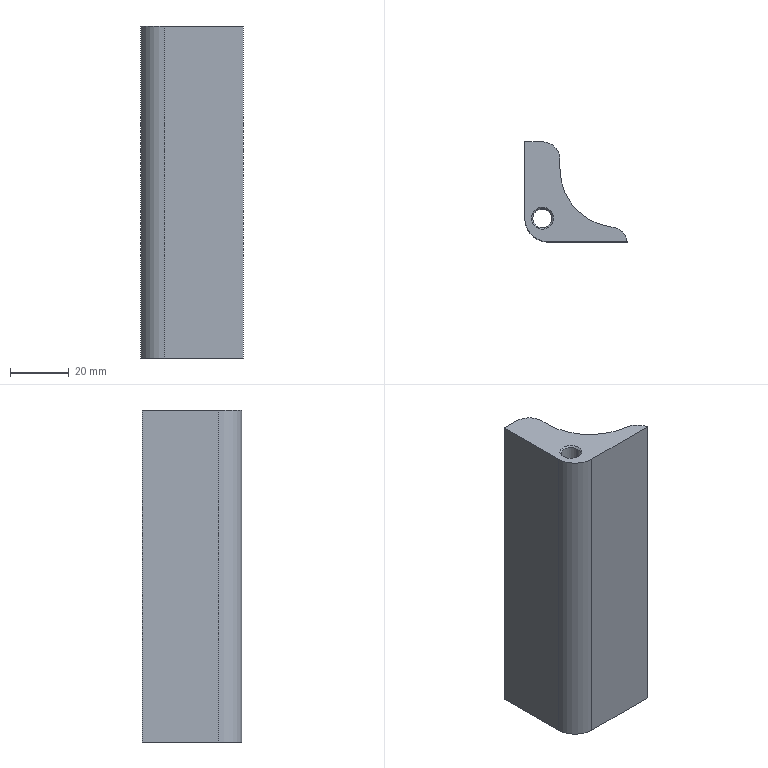Part | 1 solid | 16 faces | box 34.916 x 34 x 113 mm | volume 61391 mm3 | cylinder 6 | plane 6 | cone 4 | commonest cylinder face diameters 6.5 x2 12 x2 16 x1 40 x1
STEP:
#1=CARTESIAN_POINT('',(-3.25,9.,56.));
#2=VERTEX_POINT('',#1);
#3=CARTESIAN_POINT('',(3.25,9.,56.));
#4=VERTEX_POINT('',#3);
#5=CARTESIAN_POINT('',(0.,9.,56.));
#6=DIRECTION('',(0.,0.,1.));
#7=DIRECTION('',(1.,0.,0.));
#8=AXIS2_PLACEMENT_3D('',#5,#6,#7);
#9=CIRCLE('',#8,3.25);
#10=EDGE_CURVE('',#2,#4,#9,.T.);
#11=ORIENTED_EDGE('',*,*,#10,.F.);
#12=CARTESIAN_POINT('',(-3.75,9.,56.5));
#13=VERTEX_POINT('',#12);
#14=CARTESIAN_POINT('',(-3.25,9.,56.));
#15=DIRECTION('',(-0.7071,0.,0.7071));
#16=VECTOR('',#15,1000.);
#17=LINE('',#14,#16);
#18=EDGE_CURVE('',#2,#13,#17,.T.);
#19=ORIENTED_EDGE('',*,*,#18,.T.);
#20=CARTESIAN_POINT('',(3.75,9.,56.5));
#21=VERTEX_POINT('',#20);
#22=CARTESIAN_POINT('',(0.,9.,56.5));
#23=DIRECTION('',(0.,0.,-1.));
#24=DIRECTION('',(1.,0.,0.));
#25=AXIS2_PLACEMENT_3D('',#22,#23,#24);
#26=CIRCLE('',#25,3.75);
#27=EDGE_CURVE('',#21,#13,#26,.T.);
#28=ORIENTED_EDGE('',*,*,#27,.F.);
#29=CARTESIAN_POINT('',(3.25,9.,56.));
#30=DIRECTION('',(0.7071,0.,0.7071));
#31=VECTOR('',#30,1000.);
#32=LINE('',#29,#31);
#33=EDGE_CURVE('',#4,#21,#32,.T.);
#34=ORIENTED_EDGE('',*,*,#33,.F.);
#35=EDGE_LOOP('',(#11,#19,#28,#34));
#36=FACE_OUTER_BOUND('',#35,.T.);
#37=CARTESIAN_POINT('',(0.,9.,56.));
#38=DIRECTION('',(0.,0.,1.));
#39=DIRECTION('',(1.,0.,0.));
#40=AXIS2_PLACEMENT_3D('',#37,#38,#39);
#41=CONICAL_SURFACE('',#40,3.25,0.7854);
#42=ADVANCED_FACE('',(#36),#41,.F.);
#43=CARTESIAN_POINT('',(3.25,9.,-56.));
#44=VERTEX_POINT('',#43);
#45=CARTESIAN_POINT('',(-3.25,9.,-56.));
#46=VERTEX_POINT('',#45);
#47=CARTESIAN_POINT('',(0.,9.,-56.));
#48=DIRECTION('',(0.,0.,-1.));
#49=DIRECTION('',(1.,0.,0.));
#50=AXIS2_PLACEMENT_3D('',#47,#48,#49);
#51=CIRCLE('',#50,3.25);
#52=EDGE_CURVE('',#44,#46,#51,.T.);
#53=ORIENTED_EDGE('',*,*,#52,.F.);
#54=CARTESIAN_POINT('',(3.75,9.,-56.5));
#55=VERTEX_POINT('',#54);
#56=CARTESIAN_POINT('',(3.75,9.,-56.5));
#57=DIRECTION('',(0.7071,0.,-0.7071));
#58=VECTOR('',#57,1000.);
#59=LINE('',#56,#58);
#60=EDGE_CURVE('',#44,#55,#59,.T.);
#61=ORIENTED_EDGE('',*,*,#60,.T.);
#62=CARTESIAN_POINT('',(-3.75,9.,-56.5));
#63=VERTEX_POINT('',#62);
#64=CARTESIAN_POINT('',(0.,9.,-56.5));
#65=DIRECTION('',(0.,0.,1.));
#66=DIRECTION('',(1.,0.,0.));
#67=AXIS2_PLACEMENT_3D('',#64,#65,#66);
#68=CIRCLE('',#67,3.75);
#69=EDGE_CURVE('',#63,#55,#68,.T.);
#70=ORIENTED_EDGE('',*,*,#69,.F.);
#71=CARTESIAN_POINT('',(-3.75,9.,-56.5));
#72=DIRECTION('',(-0.7071,0.,-0.7071));
#73=VECTOR('',#72,1000.);
#74=LINE('',#71,#73);
#75=EDGE_CURVE('',#46,#63,#74,.T.);
#76=ORIENTED_EDGE('',*,*,#75,.F.);
#77=EDGE_LOOP('',(#53,#61,#70,#76));
#78=FACE_OUTER_BOUND('',#77,.T.);
#79=CARTESIAN_POINT('',(0.,9.,-56.5));
#80=DIRECTION('',(0.,0.,-1.));
#81=DIRECTION('',(-1.,0.,0.));
#82=AXIS2_PLACEMENT_3D('',#79,#80,#81);
#83=CONICAL_SURFACE('',#82,3.75,0.7854);
#84=ADVANCED_FACE('',(#78),#83,.F.);
#85=ORIENTED_EDGE('',*,*,#10,.T.);
#86=CARTESIAN_POINT('',(3.25,9.,56.5));
#87=DIRECTION('',(0.,0.,-1.));
#88=VECTOR('',#87,1000.);
#89=LINE('',#86,#88);
#90=EDGE_CURVE('',#4,#44,#89,.T.);
#91=ORIENTED_EDGE('',*,*,#90,.T.);
#92=ORIENTED_EDGE('',*,*,#52,.T.);
#93=CARTESIAN_POINT('',(-3.25,9.,56.5));
#94=DIRECTION('',(0.,0.,-1.));
#95=VECTOR('',#94,1000.);
#96=LINE('',#93,#95);
#97=EDGE_CURVE('',#2,#46,#96,.T.);
#98=ORIENTED_EDGE('',*,*,#97,.F.);
#99=EDGE_LOOP('',(#85,#91,#92,#98));
#100=FACE_OUTER_BOUND('',#99,.T.);
#101=CARTESIAN_POINT('',(0.,9.,56.5));
#102=DIRECTION('',(0.,0.,-1.));
#103=DIRECTION('',(-1.,0.,0.));
#104=AXIS2_PLACEMENT_3D('',#101,#102,#103);
#105=CYLINDRICAL_SURFACE('',#104,3.25);
#106=ADVANCED_FACE('',(#100),#105,.F.);
#107=CARTESIAN_POINT('',(-6.,35.,56.5));
#108=VERTEX_POINT('',#107);
#109=CARTESIAN_POINT('',(-6.,9.,56.5));
#110=VERTEX_POINT('',#109);
#111=CARTESIAN_POINT('',(-6.,35.,56.5));
#112=DIRECTION('',(0.,-1.,0.));
#113=VECTOR('',#112,1000.);
#114=LINE('',#111,#113);
#115=EDGE_CURVE('',#108,#110,#114,.T.);
#116=ORIENTED_EDGE('',*,*,#115,.T.);
#117=CARTESIAN_POINT('',(2.,1.,56.5));
#118=VERTEX_POINT('',#117);
#119=CARTESIAN_POINT('',(2.,9.,56.5));
#120=DIRECTION('',(0.,0.,1.));
#121=DIRECTION('',(1.,0.,0.));
#122=AXIS2_PLACEMENT_3D('',#119,#120,#121);
#123=CIRCLE('',#122,8.);
#124=EDGE_CURVE('',#110,#118,#123,.T.);
#125=ORIENTED_EDGE('',*,*,#124,.T.);
#126=CARTESIAN_POINT('',(28.916,1.,56.5));
#127=VERTEX_POINT('',#126);
#128=CARTESIAN_POINT('',(-7.315,1.,56.5));
#129=DIRECTION('',(-1.,0.,0.));
#130=VECTOR('',#129,1000.);
#131=LINE('',#128,#130);
#132=EDGE_CURVE('',#127,#118,#131,.T.);
#133=ORIENTED_EDGE('',*,*,#132,.F.);
#134=CARTESIAN_POINT('',(23.692,5.96,56.5));
#135=VERTEX_POINT('',#134);
#136=CARTESIAN_POINT('',(23.,0.,56.5));
#137=DIRECTION('',(0.,0.,1.));
#138=DIRECTION('',(1.,0.,0.));
#139=AXIS2_PLACEMENT_3D('',#136,#137,#138);
#140=CIRCLE('',#139,6.);
#141=EDGE_CURVE('',#127,#135,#140,.T.);
#142=ORIENTED_EDGE('',*,*,#141,.T.);
#143=CARTESIAN_POINT('',(6.,25.826,56.5));
#144=VERTEX_POINT('',#143);
#145=CARTESIAN_POINT('',(26.,25.826,56.5));
#146=DIRECTION('',(0.,0.,-1.));
#147=DIRECTION('',(1.,0.,0.));
#148=AXIS2_PLACEMENT_3D('',#145,#146,#147);
#149=CIRCLE('',#148,20.);
#150=EDGE_CURVE('',#135,#144,#149,.T.);
#151=ORIENTED_EDGE('',*,*,#150,.T.);
#152=CARTESIAN_POINT('',(6.,29.,56.5));
#153=VERTEX_POINT('',#152);
#154=CARTESIAN_POINT('',(6.,29.,56.5));
#155=DIRECTION('',(0.,1.,0.));
#156=VECTOR('',#155,1000.);
#157=LINE('',#154,#156);
#158=EDGE_CURVE('',#144,#153,#157,.T.);
#159=ORIENTED_EDGE('',*,*,#158,.T.);
#160=CARTESIAN_POINT('',(0.,35.,56.5));
#161=VERTEX_POINT('',#160);
#162=CARTESIAN_POINT('',(0.,29.,56.5));
#163=DIRECTION('',(0.,0.,1.));
#164=DIRECTION('',(1.,0.,0.));
#165=AXIS2_PLACEMENT_3D('',#162,#163,#164);
#166=CIRCLE('',#165,6.);
#167=EDGE_CURVE('',#153,#161,#166,.T.);
#168=ORIENTED_EDGE('',*,*,#167,.T.);
#169=CARTESIAN_POINT('',(-6.,35.,56.5));
#170=DIRECTION('',(-1.,0.,0.));
#171=VECTOR('',#170,1000.);
#172=LINE('',#169,#171);
#173=EDGE_CURVE('',#161,#108,#172,.T.);
#174=ORIENTED_EDGE('',*,*,#173,.T.);
#175=EDGE_LOOP('',(#116,#125,#133,#142,#151,#159,#168,#174));
#176=FACE_OUTER_BOUND('',#175,.T.);
#177=ORIENTED_EDGE('',*,*,#27,.T.);
#178=CARTESIAN_POINT('',(0.,9.,56.5));
#179=DIRECTION('',(0.,0.,-1.));
#180=DIRECTION('',(1.,0.,0.));
#181=AXIS2_PLACEMENT_3D('',#178,#179,#180);
#182=CIRCLE('',#181,3.75);
#183=EDGE_CURVE('',#13,#21,#182,.T.);
#184=ORIENTED_EDGE('',*,*,#183,.T.);
#185=EDGE_LOOP('',(#177,#184));
#186=FACE_BOUND('',#185,.T.);
#187=CARTESIAN_POINT('',(23.,0.,56.5));
#188=DIRECTION('',(0.,0.,1.));
#189=DIRECTION('',(1.,0.,0.));
#190=AXIS2_PLACEMENT_3D('',#187,#188,#189);
#191=PLANE('',#190);
#192=ADVANCED_FACE('',(#176,#186),#191,.T.);
#193=ORIENTED_EDGE('',*,*,#69,.T.);
#194=CARTESIAN_POINT('',(0.,9.,-56.5));
#195=DIRECTION('',(0.,0.,1.));
#196=DIRECTION('',(1.,0.,0.));
#197=AXIS2_PLACEMENT_3D('',#194,#195,#196);
#198=CIRCLE('',#197,3.75);
#199=EDGE_CURVE('',#55,#63,#198,.T.);
#200=ORIENTED_EDGE('',*,*,#199,.T.);
#201=EDGE_LOOP('',(#193,#200));
#202=FACE_BOUND('',#201,.T.);
#203=CARTESIAN_POINT('',(28.916,1.,-56.5));
#204=VERTEX_POINT('',#203);
#205=CARTESIAN_POINT('',(2.,1.,-56.5));
#206=VERTEX_POINT('',#205);
#207=CARTESIAN_POINT('',(-7.315,1.,-56.5));
#208=DIRECTION('',(-1.,0.,0.));
#209=VECTOR('',#208,1000.);
#210=LINE('',#207,#209);
#211=EDGE_CURVE('',#204,#206,#210,.T.);
#212=ORIENTED_EDGE('',*,*,#211,.T.);
#213=CARTESIAN_POINT('',(-6.,9.,-56.5));
#214=VERTEX_POINT('',#213);
#215=CARTESIAN_POINT('',(2.,9.,-56.5));
#216=DIRECTION('',(0.,0.,-1.));
#217=DIRECTION('',(1.,0.,0.));
#218=AXIS2_PLACEMENT_3D('',#215,#216,#217);
#219=CIRCLE('',#218,8.);
#220=EDGE_CURVE('',#206,#214,#219,.T.);
#221=ORIENTED_EDGE('',*,*,#220,.T.);
#222=CARTESIAN_POINT('',(-6.,35.,-56.5));
#223=VERTEX_POINT('',#222);
#224=CARTESIAN_POINT('',(-6.,35.,-56.5));
#225=DIRECTION('',(0.,-1.,0.));
#226=VECTOR('',#225,1000.);
#227=LINE('',#224,#226);
#228=EDGE_CURVE('',#223,#214,#227,.T.);
#229=ORIENTED_EDGE('',*,*,#228,.F.);
#230=CARTESIAN_POINT('',(0.,35.,-56.5));
#231=VERTEX_POINT('',#230);
#232=CARTESIAN_POINT('',(-6.,35.,-56.5));
#233=DIRECTION('',(-1.,0.,0.));
#234=VECTOR('',#233,1000.);
#235=LINE('',#232,#234);
#236=EDGE_CURVE('',#231,#223,#235,.T.);
#237=ORIENTED_EDGE('',*,*,#236,.F.);
#238=CARTESIAN_POINT('',(6.,29.,-56.5));
#239=VERTEX_POINT('',#238);
#240=CARTESIAN_POINT('',(0.,29.,-56.5));
#241=DIRECTION('',(0.,0.,1.));
#242=DIRECTION('',(1.,0.,0.));
#243=AXIS2_PLACEMENT_3D('',#240,#241,#242);
#244=CIRCLE('',#243,6.);
#245=EDGE_CURVE('',#239,#231,#244,.T.);
#246=ORIENTED_EDGE('',*,*,#245,.F.);
#247=CARTESIAN_POINT('',(6.,25.826,-56.5));
#248=VERTEX_POINT('',#247);
#249=CARTESIAN_POINT('',(6.,29.,-56.5));
#250=DIRECTION('',(0.,1.,0.));
#251=VECTOR('',#250,1000.);
#252=LINE('',#249,#251);
#253=EDGE_CURVE('',#248,#239,#252,.T.);
#254=ORIENTED_EDGE('',*,*,#253,.F.);
#255=CARTESIAN_POINT('',(23.692,5.96,-56.5));
#256=VERTEX_POINT('',#255);
#257=CARTESIAN_POINT('',(26.,25.826,-56.5));
#258=DIRECTION('',(0.,0.,1.));
#259=DIRECTION('',(1.,0.,0.));
#260=AXIS2_PLACEMENT_3D('',#257,#258,#259);
#261=CIRCLE('',#260,20.);
#262=EDGE_CURVE('',#248,#256,#261,.T.);
#263=ORIENTED_EDGE('',*,*,#262,.T.);
#264=CARTESIAN_POINT('',(23.,0.,-56.5));
#265=DIRECTION('',(0.,0.,1.));
#266=DIRECTION('',(1.,0.,0.));
#267=AXIS2_PLACEMENT_3D('',#264,#265,#266);
#268=CIRCLE('',#267,6.);
#269=EDGE_CURVE('',#204,#256,#268,.T.);
#270=ORIENTED_EDGE('',*,*,#269,.F.);
#271=EDGE_LOOP('',(#212,#221,#229,#237,#246,#254,#263,#270));
#272=FACE_OUTER_BOUND('',#271,.T.);
#273=CARTESIAN_POINT('',(23.,0.,-56.5));
#274=DIRECTION('',(0.,0.,1.));
#275=DIRECTION('',(1.,0.,0.));
#276=AXIS2_PLACEMENT_3D('',#273,#274,#275);
#277=PLANE('',#276);
#278=ADVANCED_FACE('',(#202,#272),#277,.F.);
#279=ORIENTED_EDGE('',*,*,#228,.T.);
#280=CARTESIAN_POINT('',(-6.,9.,56.5));
#281=DIRECTION('',(0.,0.,1.));
#282=VECTOR('',#281,1000.);
#283=LINE('',#280,#282);
#284=EDGE_CURVE('',#214,#110,#283,.T.);
#285=ORIENTED_EDGE('',*,*,#284,.T.);
#286=ORIENTED_EDGE('',*,*,#115,.F.);
#287=CARTESIAN_POINT('',(-6.,35.,56.5));
#288=DIRECTION('',(0.,0.,-1.));
#289=VECTOR('',#288,1000.);
#290=LINE('',#287,#289);
#291=EDGE_CURVE('',#108,#223,#290,.T.);
#292=ORIENTED_EDGE('',*,*,#291,.T.);
#293=EDGE_LOOP('',(#279,#285,#286,#292));
#294=FACE_OUTER_BOUND('',#293,.T.);
#295=CARTESIAN_POINT('',(-6.,35.,56.5));
#296=DIRECTION('',(1.,0.,0.));
#297=DIRECTION('',(0.,1.,0.));
#298=AXIS2_PLACEMENT_3D('',#295,#296,#297);
#299=PLANE('',#298);
#300=ADVANCED_FACE('',(#294),#299,.F.);
#301=ORIENTED_EDGE('',*,*,#269,.T.);
#302=CARTESIAN_POINT('',(23.692,5.96,56.5));
#303=DIRECTION('',(0.,0.,1.));
#304=VECTOR('',#303,1000.);
#305=LINE('',#302,#304);
#306=EDGE_CURVE('',#256,#135,#305,.T.);
#307=ORIENTED_EDGE('',*,*,#306,.T.);
#308=ORIENTED_EDGE('',*,*,#141,.F.);
#309=CARTESIAN_POINT('',(28.916,1.,56.5));
#310=DIRECTION('',(0.,0.,-1.));
#311=VECTOR('',#310,1000.);
#312=LINE('',#309,#311);
#313=EDGE_CURVE('',#127,#204,#312,.T.);
#314=ORIENTED_EDGE('',*,*,#313,.T.);
#315=EDGE_LOOP('',(#301,#307,#308,#314));
#316=FACE_OUTER_BOUND('',#315,.T.);
#317=CARTESIAN_POINT('',(23.,0.,56.5));
#318=DIRECTION('',(0.,0.,-1.));
#319=DIRECTION('',(-1.,0.,0.));
#320=AXIS2_PLACEMENT_3D('',#317,#318,#319);
#321=CYLINDRICAL_SURFACE('',#320,6.);
#322=ADVANCED_FACE('',(#316),#321,.T.);
#323=ORIENTED_EDGE('',*,*,#158,.F.);
#324=CARTESIAN_POINT('',(6.,25.826,-56.5));
#325=DIRECTION('',(0.,0.,-1.));
#326=VECTOR('',#325,1000.);
#327=LINE('',#324,#326);
#328=EDGE_CURVE('',#144,#248,#327,.T.);
#329=ORIENTED_EDGE('',*,*,#328,.T.);
#330=ORIENTED_EDGE('',*,*,#253,.T.);
#331=CARTESIAN_POINT('',(6.,29.,56.5));
#332=DIRECTION('',(0.,0.,-1.));
#333=VECTOR('',#332,1000.);
#334=LINE('',#331,#333);
#335=EDGE_CURVE('',#153,#239,#334,.T.);
#336=ORIENTED_EDGE('',*,*,#335,.F.);
#337=EDGE_LOOP('',(#323,#329,#330,#336));
#338=FACE_OUTER_BOUND('',#337,.T.);
#339=CARTESIAN_POINT('',(6.,29.,56.5));
#340=DIRECTION('',(-1.,0.,0.));
#341=DIRECTION('',(0.,-1.,0.));
#342=AXIS2_PLACEMENT_3D('',#339,#340,#341);
#343=PLANE('',#342);
#344=ADVANCED_FACE('',(#338),#343,.F.);
#345=ORIENTED_EDGE('',*,*,#245,.T.);
#346=CARTESIAN_POINT('',(0.,35.,56.5));
#347=DIRECTION('',(0.,0.,-1.));
#348=VECTOR('',#347,1000.);
#349=LINE('',#346,#348);
#350=EDGE_CURVE('',#161,#231,#349,.T.);
#351=ORIENTED_EDGE('',*,*,#350,.F.);
#352=ORIENTED_EDGE('',*,*,#167,.F.);
#353=ORIENTED_EDGE('',*,*,#335,.T.);
#354=EDGE_LOOP('',(#345,#351,#352,#353));
#355=FACE_OUTER_BOUND('',#354,.T.);
#356=CARTESIAN_POINT('',(0.,29.,56.5));
#357=DIRECTION('',(0.,0.,-1.));
#358=DIRECTION('',(-1.,0.,0.));
#359=AXIS2_PLACEMENT_3D('',#356,#357,#358);
#360=CYLINDRICAL_SURFACE('',#359,6.);
#361=ADVANCED_FACE('',(#355),#360,.T.);
#362=ORIENTED_EDGE('',*,*,#236,.T.);
#363=ORIENTED_EDGE('',*,*,#291,.F.);
#364=ORIENTED_EDGE('',*,*,#173,.F.);
#365=ORIENTED_EDGE('',*,*,#350,.T.);
#366=EDGE_LOOP('',(#362,#363,#364,#365));
#367=FACE_OUTER_BOUND('',#366,.T.);
#368=CARTESIAN_POINT('',(-6.,35.,56.5));
#369=DIRECTION('',(0.,-1.,0.));
#370=DIRECTION('',(1.,0.,0.));
#371=AXIS2_PLACEMENT_3D('',#368,#369,#370);
#372=PLANE('',#371);
#373=ADVANCED_FACE('',(#367),#372,.F.);
#374=ORIENTED_EDGE('',*,*,#90,.F.);
#375=CARTESIAN_POINT('',(0.,9.,56.));
#376=DIRECTION('',(0.,0.,1.));
#377=DIRECTION('',(1.,0.,0.));
#378=AXIS2_PLACEMENT_3D('',#375,#376,#377);
#379=CIRCLE('',#378,3.25);
#380=EDGE_CURVE('',#4,#2,#379,.T.);
#381=ORIENTED_EDGE('',*,*,#380,.T.);
#382=ORIENTED_EDGE('',*,*,#97,.T.);
#383=CARTESIAN_POINT('',(0.,9.,-56.));
#384=DIRECTION('',(0.,0.,-1.));
#385=DIRECTION('',(1.,0.,0.));
#386=AXIS2_PLACEMENT_3D('',#383,#384,#385);
#387=CIRCLE('',#386,3.25);
#388=EDGE_CURVE('',#46,#44,#387,.T.);
#389=ORIENTED_EDGE('',*,*,#388,.T.);
#390=EDGE_LOOP('',(#374,#381,#382,#389));
#391=FACE_OUTER_BOUND('',#390,.T.);
#392=CARTESIAN_POINT('',(0.,9.,56.5));
#393=DIRECTION('',(0.,0.,-1.));
#394=DIRECTION('',(-1.,0.,0.));
#395=AXIS2_PLACEMENT_3D('',#392,#393,#394);
#396=CYLINDRICAL_SURFACE('',#395,3.25);
#397=ADVANCED_FACE('',(#391),#396,.F.);
#398=ORIENTED_EDGE('',*,*,#60,.F.);
#399=ORIENTED_EDGE('',*,*,#388,.F.);
#400=ORIENTED_EDGE('',*,*,#75,.T.);
#401=ORIENTED_EDGE('',*,*,#199,.F.);
#402=EDGE_LOOP('',(#398,#399,#400,#401));
#403=FACE_OUTER_BOUND('',#402,.T.);
#404=CARTESIAN_POINT('',(0.,9.,-56.5));
#405=DIRECTION('',(0.,0.,-1.));
#406=DIRECTION('',(-1.,0.,0.));
#407=AXIS2_PLACEMENT_3D('',#404,#405,#406);
#408=CONICAL_SURFACE('',#407,3.75,0.7854);
#409=ADVANCED_FACE('',(#403),#408,.F.);
#410=ORIENTED_EDGE('',*,*,#18,.F.);
#411=ORIENTED_EDGE('',*,*,#380,.F.);
#412=ORIENTED_EDGE('',*,*,#33,.T.);
#413=ORIENTED_EDGE('',*,*,#183,.F.);
#414=EDGE_LOOP('',(#410,#411,#412,#413));
#415=FACE_OUTER_BOUND('',#414,.T.);
#416=CARTESIAN_POINT('',(0.,9.,56.));
#417=DIRECTION('',(0.,0.,1.));
#418=DIRECTION('',(1.,0.,0.));
#419=AXIS2_PLACEMENT_3D('',#416,#417,#418);
#420=CONICAL_SURFACE('',#419,3.25,0.7854);
#421=ADVANCED_FACE('',(#415),#420,.F.);
#422=ORIENTED_EDGE('',*,*,#132,.T.);
#423=CARTESIAN_POINT('',(2.,1.,-56.5));
#424=DIRECTION('',(0.,0.,-1.));
#425=VECTOR('',#424,1000.);
#426=LINE('',#423,#425);
#427=EDGE_CURVE('',#118,#206,#426,.T.);
#428=ORIENTED_EDGE('',*,*,#427,.T.);
#429=ORIENTED_EDGE('',*,*,#211,.F.);
#430=ORIENTED_EDGE('',*,*,#313,.F.);
#431=EDGE_LOOP('',(#422,#428,#429,#430));
#432=FACE_OUTER_BOUND('',#431,.T.);
#433=CARTESIAN_POINT('',(-7.315,1.,-56.5));
#434=DIRECTION('',(0.,1.,0.));
#435=DIRECTION('',(0.,0.,1.));
#436=AXIS2_PLACEMENT_3D('',#433,#434,#435);
#437=PLANE('',#436);
#438=ADVANCED_FACE('',(#432),#437,.F.);
#439=ORIENTED_EDGE('',*,*,#150,.F.);
#440=ORIENTED_EDGE('',*,*,#306,.F.);
#441=ORIENTED_EDGE('',*,*,#262,.F.);
#442=ORIENTED_EDGE('',*,*,#328,.F.);
#443=EDGE_LOOP('',(#439,#440,#441,#442));
#444=FACE_OUTER_BOUND('',#443,.T.);
#445=CARTESIAN_POINT('',(26.,25.826,56.5));
#446=DIRECTION('',(0.,0.,-1.));
#447=DIRECTION('',(-1.,0.,0.));
#448=AXIS2_PLACEMENT_3D('',#445,#446,#447);
#449=CYLINDRICAL_SURFACE('',#448,20.);
#450=ADVANCED_FACE('',(#444),#449,.F.);
#451=ORIENTED_EDGE('',*,*,#220,.F.);
#452=ORIENTED_EDGE('',*,*,#427,.F.);
#453=ORIENTED_EDGE('',*,*,#124,.F.);
#454=ORIENTED_EDGE('',*,*,#284,.F.);
#455=EDGE_LOOP('',(#451,#452,#453,#454));
#456=FACE_OUTER_BOUND('',#455,.T.);
#457=CARTESIAN_POINT('',(2.,9.,56.5));
#458=DIRECTION('',(0.,0.,1.));
#459=DIRECTION('',(1.,0.,0.));
#460=AXIS2_PLACEMENT_3D('',#457,#458,#459);
#461=CYLINDRICAL_SURFACE('',#460,8.);
#462=ADVANCED_FACE('',(#456),#461,.T.);
#463=CLOSED_SHELL('',(#42,#84,#106,#192,#278,#300,#322,#344,#361,#373,#397,#409,#421,#438,#450,#462));
#464=MANIFOLD_SOLID_BREP('',#463);
#465=CARTESIAN_POINT('',(0.,0.,0.));
#466=DIRECTION('',(0.,0.,1.));
#467=DIRECTION('',(1.,0.,0.));
#468=AXIS2_PLACEMENT_3D('',#465,#466,#467);
#469=(LENGTH_UNIT()NAMED_UNIT(*)SI_UNIT(.MILLI.,.METRE.));
#470=UNCERTAINTY_MEASURE_WITH_UNIT(LENGTH_MEASURE(0.00001),#469,'','');
#471=(NAMED_UNIT(*)PLANE_ANGLE_UNIT()SI_UNIT($,.RADIAN.));
#472=(NAMED_UNIT(*)SI_UNIT($,.STERADIAN.)SOLID_ANGLE_UNIT());
#473=(GEOMETRIC_REPRESENTATION_CONTEXT(3)GLOBAL_UNCERTAINTY_ASSIGNED_CONTEXT((#470))GLOBAL_UNIT_ASSIGNED_CONTEXT((#469,#471,#472))REPRESENTATION_CONTEXT('',''));
#474=ADVANCED_BREP_SHAPE_REPRESENTATION('',(#464,#468),#473);